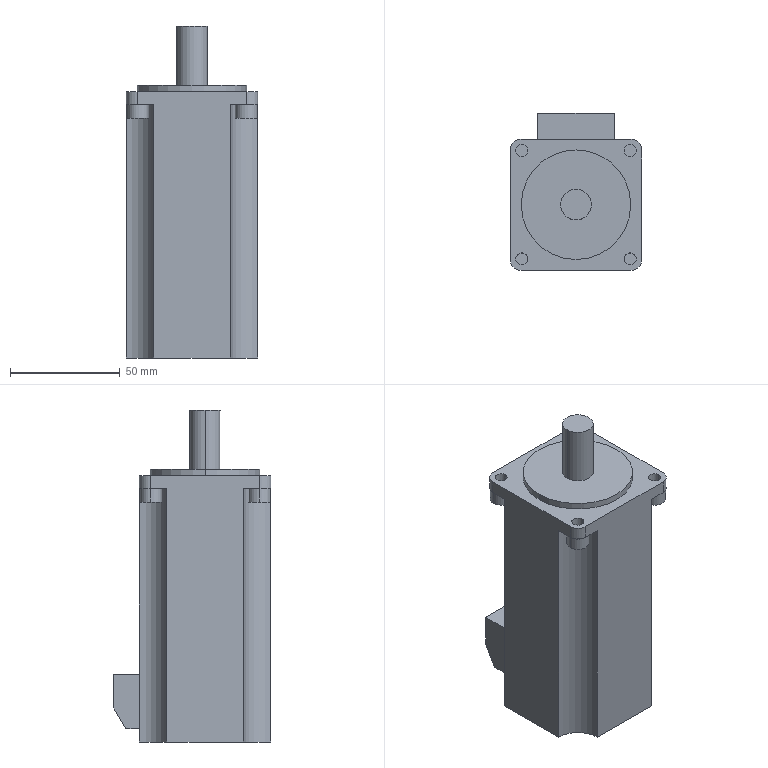Part | SolidWorks | features ICE 5, Chamfer 1, Extrusion 1, Fillet 1, HoleWzd 1 | 1 solid | 55 faces | box 60 x 72 x 151.5 mm | volume 401427 mm3 | cylinder 28 | plane 27 | commonest cylinder face diameters 10 x12 5.5 x8 25 x4 14 x2 50 x2
STEP:
#1=CARTESIAN_POINT('',(-29.749,24.749,-42.));
#2=VERTEX_POINT('',#1);
#3=CARTESIAN_POINT('',(-19.749,24.749,-42.));
#4=VERTEX_POINT('',#3);
#5=CARTESIAN_POINT('',(-24.749,24.749,-42.));
#6=DIRECTION('',(0.,0.,-1.));
#7=DIRECTION('',(-1.,0.,0.));
#8=AXIS2_PLACEMENT_3D('',#5,#6,#7);
#9=CIRCLE('',#8,5.);
#10=EDGE_CURVE('',#2,#4,#9,.T.);
#11=ORIENTED_EDGE('',*,*,#10,.F.);
#12=CARTESIAN_POINT('',(-29.749,24.749,-36.));
#13=VERTEX_POINT('',#12);
#14=CARTESIAN_POINT('',(-29.749,24.749,-42.));
#15=DIRECTION('',(0.,0.,1.));
#16=VECTOR('',#15,1000.);
#17=LINE('',#14,#16);
#18=EDGE_CURVE('',#2,#13,#17,.T.);
#19=ORIENTED_EDGE('',*,*,#18,.T.);
#20=CARTESIAN_POINT('',(-19.749,24.749,-36.));
#21=VERTEX_POINT('',#20);
#22=CARTESIAN_POINT('',(-24.749,24.749,-36.));
#23=DIRECTION('',(0.,0.,-1.));
#24=DIRECTION('',(-1.,0.,0.));
#25=AXIS2_PLACEMENT_3D('',#22,#23,#24);
#26=CIRCLE('',#25,5.);
#27=EDGE_CURVE('',#13,#21,#26,.T.);
#28=ORIENTED_EDGE('',*,*,#27,.T.);
#29=CARTESIAN_POINT('',(-19.749,24.749,-42.));
#30=DIRECTION('',(0.,0.,1.));
#31=VECTOR('',#30,1000.);
#32=LINE('',#29,#31);
#33=EDGE_CURVE('',#4,#21,#32,.T.);
#34=ORIENTED_EDGE('',*,*,#33,.F.);
#35=EDGE_LOOP('',(#11,#19,#28,#34));
#36=FACE_OUTER_BOUND('',#35,.T.);
#37=CARTESIAN_POINT('',(-24.749,24.749,-42.));
#38=DIRECTION('',(0.,0.,1.));
#39=DIRECTION('',(1.,0.,0.));
#40=AXIS2_PLACEMENT_3D('',#37,#38,#39);
#41=CYLINDRICAL_SURFACE('',#40,5.);
#42=ADVANCED_FACE('',(#36),#41,.T.);
#43=CARTESIAN_POINT('',(-29.749,-24.749,-42.));
#44=VERTEX_POINT('',#43);
#45=CARTESIAN_POINT('',(-19.749,-24.749,-42.));
#46=VERTEX_POINT('',#45);
#47=CARTESIAN_POINT('',(-24.749,-24.749,-42.));
#48=DIRECTION('',(0.,0.,-1.));
#49=DIRECTION('',(-1.,0.,0.));
#50=AXIS2_PLACEMENT_3D('',#47,#48,#49);
#51=CIRCLE('',#50,5.);
#52=EDGE_CURVE('',#44,#46,#51,.T.);
#53=ORIENTED_EDGE('',*,*,#52,.F.);
#54=CARTESIAN_POINT('',(-29.749,-24.749,-36.));
#55=VERTEX_POINT('',#54);
#56=CARTESIAN_POINT('',(-29.749,-24.749,-42.));
#57=DIRECTION('',(0.,0.,1.));
#58=VECTOR('',#57,1000.);
#59=LINE('',#56,#58);
#60=EDGE_CURVE('',#44,#55,#59,.T.);
#61=ORIENTED_EDGE('',*,*,#60,.T.);
#62=CARTESIAN_POINT('',(-19.749,-24.749,-36.));
#63=VERTEX_POINT('',#62);
#64=CARTESIAN_POINT('',(-24.749,-24.749,-36.));
#65=DIRECTION('',(0.,0.,-1.));
#66=DIRECTION('',(-1.,0.,0.));
#67=AXIS2_PLACEMENT_3D('',#64,#65,#66);
#68=CIRCLE('',#67,5.);
#69=EDGE_CURVE('',#55,#63,#68,.T.);
#70=ORIENTED_EDGE('',*,*,#69,.T.);
#71=CARTESIAN_POINT('',(-19.749,-24.749,-42.));
#72=DIRECTION('',(0.,0.,1.));
#73=VECTOR('',#72,1000.);
#74=LINE('',#71,#73);
#75=EDGE_CURVE('',#46,#63,#74,.T.);
#76=ORIENTED_EDGE('',*,*,#75,.F.);
#77=EDGE_LOOP('',(#53,#61,#70,#76));
#78=FACE_OUTER_BOUND('',#77,.T.);
#79=CARTESIAN_POINT('',(-24.749,-24.749,-42.));
#80=DIRECTION('',(0.,0.,1.));
#81=DIRECTION('',(1.,0.,0.));
#82=AXIS2_PLACEMENT_3D('',#79,#80,#81);
#83=CYLINDRICAL_SURFACE('',#82,5.);
#84=ADVANCED_FACE('',(#78),#83,.T.);
#85=CARTESIAN_POINT('',(19.749,-24.749,-42.));
#86=VERTEX_POINT('',#85);
#87=CARTESIAN_POINT('',(29.749,-24.749,-42.));
#88=VERTEX_POINT('',#87);
#89=CARTESIAN_POINT('',(24.749,-24.749,-42.));
#90=DIRECTION('',(0.,0.,-1.));
#91=DIRECTION('',(-1.,0.,0.));
#92=AXIS2_PLACEMENT_3D('',#89,#90,#91);
#93=CIRCLE('',#92,5.);
#94=EDGE_CURVE('',#86,#88,#93,.T.);
#95=ORIENTED_EDGE('',*,*,#94,.F.);
#96=CARTESIAN_POINT('',(19.749,-24.749,-36.));
#97=VERTEX_POINT('',#96);
#98=CARTESIAN_POINT('',(19.749,-24.749,-42.));
#99=DIRECTION('',(0.,0.,1.));
#100=VECTOR('',#99,1000.);
#101=LINE('',#98,#100);
#102=EDGE_CURVE('',#86,#97,#101,.T.);
#103=ORIENTED_EDGE('',*,*,#102,.T.);
#104=CARTESIAN_POINT('',(29.749,-24.749,-36.));
#105=VERTEX_POINT('',#104);
#106=CARTESIAN_POINT('',(24.749,-24.749,-36.));
#107=DIRECTION('',(0.,0.,-1.));
#108=DIRECTION('',(-1.,0.,0.));
#109=AXIS2_PLACEMENT_3D('',#106,#107,#108);
#110=CIRCLE('',#109,5.);
#111=EDGE_CURVE('',#97,#105,#110,.T.);
#112=ORIENTED_EDGE('',*,*,#111,.T.);
#113=CARTESIAN_POINT('',(29.749,-24.749,-42.));
#114=DIRECTION('',(0.,0.,1.));
#115=VECTOR('',#114,1000.);
#116=LINE('',#113,#115);
#117=EDGE_CURVE('',#88,#105,#116,.T.);
#118=ORIENTED_EDGE('',*,*,#117,.F.);
#119=EDGE_LOOP('',(#95,#103,#112,#118));
#120=FACE_OUTER_BOUND('',#119,.T.);
#121=CARTESIAN_POINT('',(24.749,-24.749,-42.));
#122=DIRECTION('',(0.,0.,1.));
#123=DIRECTION('',(1.,0.,0.));
#124=AXIS2_PLACEMENT_3D('',#121,#122,#123);
#125=CYLINDRICAL_SURFACE('',#124,5.);
#126=ADVANCED_FACE('',(#120),#125,.T.);
#127=CARTESIAN_POINT('',(19.749,24.749,-42.));
#128=VERTEX_POINT('',#127);
#129=CARTESIAN_POINT('',(29.749,24.749,-42.));
#130=VERTEX_POINT('',#129);
#131=CARTESIAN_POINT('',(24.749,24.749,-42.));
#132=DIRECTION('',(0.,0.,-1.));
#133=DIRECTION('',(-1.,0.,0.));
#134=AXIS2_PLACEMENT_3D('',#131,#132,#133);
#135=CIRCLE('',#134,5.);
#136=EDGE_CURVE('',#128,#130,#135,.T.);
#137=ORIENTED_EDGE('',*,*,#136,.F.);
#138=CARTESIAN_POINT('',(19.749,24.749,-36.));
#139=VERTEX_POINT('',#138);
#140=CARTESIAN_POINT('',(19.749,24.749,-42.));
#141=DIRECTION('',(0.,0.,1.));
#142=VECTOR('',#141,1000.);
#143=LINE('',#140,#142);
#144=EDGE_CURVE('',#128,#139,#143,.T.);
#145=ORIENTED_EDGE('',*,*,#144,.T.);
#146=CARTESIAN_POINT('',(29.749,24.749,-36.));
#147=VERTEX_POINT('',#146);
#148=CARTESIAN_POINT('',(24.749,24.749,-36.));
#149=DIRECTION('',(0.,0.,-1.));
#150=DIRECTION('',(-1.,0.,0.));
#151=AXIS2_PLACEMENT_3D('',#148,#149,#150);
#152=CIRCLE('',#151,5.);
#153=EDGE_CURVE('',#139,#147,#152,.T.);
#154=ORIENTED_EDGE('',*,*,#153,.T.);
#155=CARTESIAN_POINT('',(29.749,24.749,-42.));
#156=DIRECTION('',(0.,0.,1.));
#157=VECTOR('',#156,1000.);
#158=LINE('',#155,#157);
#159=EDGE_CURVE('',#130,#147,#158,.T.);
#160=ORIENTED_EDGE('',*,*,#159,.F.);
#161=EDGE_LOOP('',(#137,#145,#154,#160));
#162=FACE_OUTER_BOUND('',#161,.T.);
#163=CARTESIAN_POINT('',(24.749,24.749,-42.));
#164=DIRECTION('',(0.,0.,1.));
#165=DIRECTION('',(1.,0.,0.));
#166=AXIS2_PLACEMENT_3D('',#163,#164,#165);
#167=CYLINDRICAL_SURFACE('',#166,5.);
#168=ADVANCED_FACE('',(#162),#167,.T.);
#169=CARTESIAN_POINT('',(21.999,24.749,-36.));
#170=VERTEX_POINT('',#169);
#171=CARTESIAN_POINT('',(27.499,24.749,-36.));
#172=VERTEX_POINT('',#171);
#173=CARTESIAN_POINT('',(24.749,24.749,-36.));
#174=DIRECTION('',(0.,0.,1.));
#175=DIRECTION('',(-1.,0.,0.));
#176=AXIS2_PLACEMENT_3D('',#173,#174,#175);
#177=CIRCLE('',#176,2.75);
#178=EDGE_CURVE('',#170,#172,#177,.T.);
#179=ORIENTED_EDGE('',*,*,#178,.F.);
#180=CARTESIAN_POINT('',(21.999,24.749,-30.));
#181=VERTEX_POINT('',#180);
#182=CARTESIAN_POINT('',(21.999,24.749,-30.));
#183=DIRECTION('',(0.,0.,1.));
#184=VECTOR('',#183,1000.);
#185=LINE('',#182,#184);
#186=EDGE_CURVE('',#170,#181,#185,.T.);
#187=ORIENTED_EDGE('',*,*,#186,.T.);
#188=CARTESIAN_POINT('',(27.499,24.749,-30.));
#189=VERTEX_POINT('',#188);
#190=CARTESIAN_POINT('',(24.749,24.749,-30.));
#191=DIRECTION('',(0.,0.,1.));
#192=DIRECTION('',(1.,0.,0.));
#193=AXIS2_PLACEMENT_3D('',#190,#191,#192);
#194=CIRCLE('',#193,2.75);
#195=EDGE_CURVE('',#181,#189,#194,.T.);
#196=ORIENTED_EDGE('',*,*,#195,.T.);
#197=CARTESIAN_POINT('',(27.499,24.749,-30.));
#198=DIRECTION('',(0.,0.,1.));
#199=VECTOR('',#198,1000.);
#200=LINE('',#197,#199);
#201=EDGE_CURVE('',#172,#189,#200,.T.);
#202=ORIENTED_EDGE('',*,*,#201,.F.);
#203=EDGE_LOOP('',(#179,#187,#196,#202));
#204=FACE_OUTER_BOUND('',#203,.T.);
#205=CARTESIAN_POINT('',(24.749,24.749,-30.));
#206=DIRECTION('',(0.,0.,1.));
#207=DIRECTION('',(1.,0.,0.));
#208=AXIS2_PLACEMENT_3D('',#205,#206,#207);
#209=CYLINDRICAL_SURFACE('',#208,2.75);
#210=ADVANCED_FACE('',(#204),#209,.F.);
#211=CARTESIAN_POINT('',(-27.499,24.749,-36.));
#212=VERTEX_POINT('',#211);
#213=CARTESIAN_POINT('',(-21.999,24.749,-36.));
#214=VERTEX_POINT('',#213);
#215=CARTESIAN_POINT('',(-24.749,24.749,-36.));
#216=DIRECTION('',(0.,0.,1.));
#217=DIRECTION('',(-1.,0.,0.));
#218=AXIS2_PLACEMENT_3D('',#215,#216,#217);
#219=CIRCLE('',#218,2.75);
#220=EDGE_CURVE('',#212,#214,#219,.T.);
#221=ORIENTED_EDGE('',*,*,#220,.F.);
#222=CARTESIAN_POINT('',(-27.499,24.749,-30.));
#223=VERTEX_POINT('',#222);
#224=CARTESIAN_POINT('',(-27.499,24.749,-30.));
#225=DIRECTION('',(0.,0.,1.));
#226=VECTOR('',#225,1000.);
#227=LINE('',#224,#226);
#228=EDGE_CURVE('',#212,#223,#227,.T.);
#229=ORIENTED_EDGE('',*,*,#228,.T.);
#230=CARTESIAN_POINT('',(-21.999,24.749,-30.));
#231=VERTEX_POINT('',#230);
#232=CARTESIAN_POINT('',(-24.749,24.749,-30.));
#233=DIRECTION('',(0.,0.,1.));
#234=DIRECTION('',(1.,0.,0.));
#235=AXIS2_PLACEMENT_3D('',#232,#233,#234);
#236=CIRCLE('',#235,2.75);
#237=EDGE_CURVE('',#223,#231,#236,.T.);
#238=ORIENTED_EDGE('',*,*,#237,.T.);
#239=CARTESIAN_POINT('',(-21.999,24.749,-30.));
#240=DIRECTION('',(0.,0.,1.));
#241=VECTOR('',#240,1000.);
#242=LINE('',#239,#241);
#243=EDGE_CURVE('',#214,#231,#242,.T.);
#244=ORIENTED_EDGE('',*,*,#243,.F.);
#245=EDGE_LOOP('',(#221,#229,#238,#244));
#246=FACE_OUTER_BOUND('',#245,.T.);
#247=CARTESIAN_POINT('',(-24.749,24.749,-30.));
#248=DIRECTION('',(0.,0.,1.));
#249=DIRECTION('',(1.,0.,0.));
#250=AXIS2_PLACEMENT_3D('',#247,#248,#249);
#251=CYLINDRICAL_SURFACE('',#250,2.75);
#252=ADVANCED_FACE('',(#246),#251,.F.);
#253=CARTESIAN_POINT('',(21.999,-24.749,-36.));
#254=VERTEX_POINT('',#253);
#255=CARTESIAN_POINT('',(27.499,-24.749,-36.));
#256=VERTEX_POINT('',#255);
#257=CARTESIAN_POINT('',(24.749,-24.749,-36.));
#258=DIRECTION('',(0.,0.,1.));
#259=DIRECTION('',(-1.,0.,0.));
#260=AXIS2_PLACEMENT_3D('',#257,#258,#259);
#261=CIRCLE('',#260,2.75);
#262=EDGE_CURVE('',#254,#256,#261,.T.);
#263=ORIENTED_EDGE('',*,*,#262,.F.);
#264=CARTESIAN_POINT('',(21.999,-24.749,-30.));
#265=VERTEX_POINT('',#264);
#266=CARTESIAN_POINT('',(21.999,-24.749,-30.));
#267=DIRECTION('',(0.,0.,1.));
#268=VECTOR('',#267,1000.);
#269=LINE('',#266,#268);
#270=EDGE_CURVE('',#254,#265,#269,.T.);
#271=ORIENTED_EDGE('',*,*,#270,.T.);
#272=CARTESIAN_POINT('',(27.499,-24.749,-30.));
#273=VERTEX_POINT('',#272);
#274=CARTESIAN_POINT('',(24.749,-24.749,-30.));
#275=DIRECTION('',(0.,0.,1.));
#276=DIRECTION('',(1.,0.,0.));
#277=AXIS2_PLACEMENT_3D('',#274,#275,#276);
#278=CIRCLE('',#277,2.75);
#279=EDGE_CURVE('',#265,#273,#278,.T.);
#280=ORIENTED_EDGE('',*,*,#279,.T.);
#281=CARTESIAN_POINT('',(27.499,-24.749,-30.));
#282=DIRECTION('',(0.,0.,1.));
#283=VECTOR('',#282,1000.);
#284=LINE('',#281,#283);
#285=EDGE_CURVE('',#256,#273,#284,.T.);
#286=ORIENTED_EDGE('',*,*,#285,.F.);
#287=EDGE_LOOP('',(#263,#271,#280,#286));
#288=FACE_OUTER_BOUND('',#287,.T.);
#289=CARTESIAN_POINT('',(24.749,-24.749,-30.));
#290=DIRECTION('',(0.,0.,1.));
#291=DIRECTION('',(1.,0.,0.));
#292=AXIS2_PLACEMENT_3D('',#289,#290,#291);
#293=CYLINDRICAL_SURFACE('',#292,2.75);
#294=ADVANCED_FACE('',(#288),#293,.F.);
#295=CARTESIAN_POINT('',(-27.499,-24.749,-36.));
#296=VERTEX_POINT('',#295);
#297=CARTESIAN_POINT('',(-21.999,-24.749,-36.));
#298=VERTEX_POINT('',#297);
#299=CARTESIAN_POINT('',(-24.749,-24.749,-36.));
#300=DIRECTION('',(0.,0.,1.));
#301=DIRECTION('',(-1.,0.,0.));
#302=AXIS2_PLACEMENT_3D('',#299,#300,#301);
#303=CIRCLE('',#302,2.75);
#304=EDGE_CURVE('',#296,#298,#303,.T.);
#305=ORIENTED_EDGE('',*,*,#304,.F.);
#306=CARTESIAN_POINT('',(-27.499,-24.749,-30.));
#307=VERTEX_POINT('',#306);
#308=CARTESIAN_POINT('',(-27.499,-24.749,-30.));
#309=DIRECTION('',(0.,0.,1.));
#310=VECTOR('',#309,1000.);
#311=LINE('',#308,#310);
#312=EDGE_CURVE('',#296,#307,#311,.T.);
#313=ORIENTED_EDGE('',*,*,#312,.T.);
#314=CARTESIAN_POINT('',(-21.999,-24.749,-30.));
#315=VERTEX_POINT('',#314);
#316=CARTESIAN_POINT('',(-24.749,-24.749,-30.));
#317=DIRECTION('',(0.,0.,1.));
#318=DIRECTION('',(1.,0.,0.));
#319=AXIS2_PLACEMENT_3D('',#316,#317,#318);
#320=CIRCLE('',#319,2.75);
#321=EDGE_CURVE('',#307,#315,#320,.T.);
#322=ORIENTED_EDGE('',*,*,#321,.T.);
#323=CARTESIAN_POINT('',(-21.999,-24.749,-30.));
#324=DIRECTION('',(0.,0.,1.));
#325=VECTOR('',#324,1000.);
#326=LINE('',#323,#325);
#327=EDGE_CURVE('',#298,#315,#326,.T.);
#328=ORIENTED_EDGE('',*,*,#327,.F.);
#329=EDGE_LOOP('',(#305,#313,#322,#328));
#330=FACE_OUTER_BOUND('',#329,.T.);
#331=CARTESIAN_POINT('',(-24.749,-24.749,-30.));
#332=DIRECTION('',(0.,0.,1.));
#333=DIRECTION('',(1.,0.,0.));
#334=AXIS2_PLACEMENT_3D('',#331,#332,#333);
#335=CYLINDRICAL_SURFACE('',#334,2.75);
#336=ADVANCED_FACE('',(#330),#335,.F.);
#337=CARTESIAN_POINT('',(-25.,0.,-27.));
#338=VERTEX_POINT('',#337);
#339=CARTESIAN_POINT('',(25.,0.,-27.));
#340=VERTEX_POINT('',#339);
#341=CARTESIAN_POINT('',(0.,0.,-27.));
#342=DIRECTION('',(0.,0.,-1.));
#343=DIRECTION('',(-1.,0.,0.));
#344=AXIS2_PLACEMENT_3D('',#341,#342,#343);
#345=CIRCLE('',#344,25.);
#346=EDGE_CURVE('',#338,#340,#345,.T.);
#347=ORIENTED_EDGE('',*,*,#346,.T.);
#348=CARTESIAN_POINT('',(25.,0.,-30.));
#349=VERTEX_POINT('',#348);
#350=CARTESIAN_POINT('',(25.,0.,-27.));
#351=DIRECTION('',(0.,0.,-1.));
#352=VECTOR('',#351,1000.);
#353=LINE('',#350,#352);
#354=EDGE_CURVE('',#340,#349,#353,.T.);
#355=ORIENTED_EDGE('',*,*,#354,.T.);
#356=CARTESIAN_POINT('',(-25.,0.,-30.));
#357=VERTEX_POINT('',#356);
#358=CARTESIAN_POINT('',(0.,0.,-30.));
#359=DIRECTION('',(0.,0.,-1.));
#360=DIRECTION('',(-1.,0.,0.));
#361=AXIS2_PLACEMENT_3D('',#358,#359,#360);
#362=CIRCLE('',#361,25.);
#363=EDGE_CURVE('',#357,#349,#362,.T.);
#364=ORIENTED_EDGE('',*,*,#363,.F.);
#365=CARTESIAN_POINT('',(-25.,0.,-27.));
#366=DIRECTION('',(0.,0.,-1.));
#367=VECTOR('',#366,1000.);
#368=LINE('',#365,#367);
#369=EDGE_CURVE('',#338,#357,#368,.T.);
#370=ORIENTED_EDGE('',*,*,#369,.F.);
#371=EDGE_LOOP('',(#347,#355,#364,#370));
#372=FACE_OUTER_BOUND('',#371,.T.);
#373=CARTESIAN_POINT('',(0.,0.,-27.));
#374=DIRECTION('',(0.,0.,-1.));
#375=DIRECTION('',(-1.,0.,0.));
#376=AXIS2_PLACEMENT_3D('',#373,#374,#375);
#377=CYLINDRICAL_SURFACE('',#376,25.);
#378=ADVANCED_FACE('',(#372),#377,.T.);
#379=CARTESIAN_POINT('',(7.,0.,-27.));
#380=VERTEX_POINT('',#379);
#381=CARTESIAN_POINT('',(-7.,0.,-27.));
#382=VERTEX_POINT('',#381);
#383=CARTESIAN_POINT('',(0.,0.,-27.));
#384=DIRECTION('',(0.,0.,1.));
#385=DIRECTION('',(-1.,0.,0.));
#386=AXIS2_PLACEMENT_3D('',#383,#384,#385);
#387=CIRCLE('',#386,7.);
#388=EDGE_CURVE('',#380,#382,#387,.T.);
#389=ORIENTED_EDGE('',*,*,#388,.T.);
#390=CARTESIAN_POINT('',(-7.,0.,0.));
#391=VERTEX_POINT('',#390);
#392=CARTESIAN_POINT('',(-7.,0.,-30.));
#393=DIRECTION('',(0.,0.,1.));
#394=VECTOR('',#393,1000.);
#395=LINE('',#392,#394);
#396=EDGE_CURVE('',#382,#391,#395,.T.);
#397=ORIENTED_EDGE('',*,*,#396,.T.);
#398=CARTESIAN_POINT('',(7.,0.,0.));
#399=VERTEX_POINT('',#398);
#400=CARTESIAN_POINT('',(0.,0.,0.));
#401=DIRECTION('',(0.,0.,1.));
#402=DIRECTION('',(1.,0.,0.));
#403=AXIS2_PLACEMENT_3D('',#400,#401,#402);
#404=CIRCLE('',#403,7.);
#405=EDGE_CURVE('',#399,#391,#404,.T.);
#406=ORIENTED_EDGE('',*,*,#405,.F.);
#407=CARTESIAN_POINT('',(7.,0.,-30.));
#408=DIRECTION('',(0.,0.,1.));
#409=VECTOR('',#408,1000.);
#410=LINE('',#407,#409);
#411=EDGE_CURVE('',#380,#399,#410,.T.);
#412=ORIENTED_EDGE('',*,*,#411,.F.);
#413=EDGE_LOOP('',(#389,#397,#406,#412));
#414=FACE_OUTER_BOUND('',#413,.T.);
#415=CARTESIAN_POINT('',(0.,0.,-30.));
#416=DIRECTION('',(0.,0.,1.));
#417=DIRECTION('',(1.,0.,0.));
#418=AXIS2_PLACEMENT_3D('',#415,#416,#417);
#419=CYLINDRICAL_SURFACE('',#418,7.);
#420=ADVANCED_FACE('',(#414),#419,.T.);
#421=CARTESIAN_POINT('',(-30.,17.5,-36.));
#422=VERTEX_POINT('',#421);
#423=CARTESIAN_POINT('',(-30.,25.,-36.));
#424=VERTEX_POINT('',#423);
#425=CARTESIAN_POINT('',(-30.,30.,-36.));
#426=DIRECTION('',(0.,1.,0.));
#427=VECTOR('',#426,1000.);
#428=LINE('',#425,#427);
#429=EDGE_CURVE('',#422,#424,#428,.T.);
#430=ORIENTED_EDGE('',*,*,#429,.T.);
#431=CARTESIAN_POINT('',(-25.,30.,-36.));
#432=VERTEX_POINT('',#431);
#433=CARTESIAN_POINT('',(-25.,25.,-36.));
#434=DIRECTION('',(0.,0.,-1.));
#435=DIRECTION('',(-1.,0.,0.));
#436=AXIS2_PLACEMENT_3D('',#433,#434,#435);
#437=CIRCLE('',#436,5.);
#438=EDGE_CURVE('',#424,#432,#437,.T.);
#439=ORIENTED_EDGE('',*,*,#438,.T.);
#440=CARTESIAN_POINT('',(-17.5,30.,-36.));
#441=VERTEX_POINT('',#440);
#442=CARTESIAN_POINT('',(30.,30.,-36.));
#443=DIRECTION('',(1.,0.,0.));
#444=VECTOR('',#443,1000.);
#445=LINE('',#442,#444);
#446=EDGE_CURVE('',#432,#441,#445,.T.);
#447=ORIENTED_EDGE('',*,*,#446,.T.);
#448=CARTESIAN_POINT('',(-30.,30.,-36.));
#449=DIRECTION('',(0.,0.,1.));
#450=DIRECTION('',(-1.,0.,0.));
#451=AXIS2_PLACEMENT_3D('',#448,#449,#450);
#452=CIRCLE('',#451,12.5);
#453=EDGE_CURVE('',#422,#441,#452,.T.);
#454=ORIENTED_EDGE('',*,*,#453,.F.);
#455=EDGE_LOOP('',(#430,#439,#447,#454));
#456=FACE_OUTER_BOUND('',#455,.T.);
#457=CARTESIAN_POINT('',(-24.749,24.749,-36.));
#458=DIRECTION('',(0.,0.,-1.));
#459=DIRECTION('',(-1.,0.,0.));
#460=AXIS2_PLACEMENT_3D('',#457,#458,#459);
#461=CIRCLE('',#460,5.);
#462=EDGE_CURVE('',#21,#13,#461,.T.);
#463=ORIENTED_EDGE('',*,*,#462,.F.);
#464=ORIENTED_EDGE('',*,*,#27,.F.);
#465=EDGE_LOOP('',(#463,#464));
#466=FACE_BOUND('',#465,.T.);
#467=CARTESIAN_POINT('',(0.,0.,-36.));
#468=DIRECTION('',(0.,0.,-1.));
#469=DIRECTION('',(-1.,0.,0.));
#470=AXIS2_PLACEMENT_3D('',#467,#468,#469);
#471=PLANE('',#470);
#472=ADVANCED_FACE('',(#456,#466),#471,.T.);
#473=CARTESIAN_POINT('',(-17.5,-30.,-36.));
#474=VERTEX_POINT('',#473);
#475=CARTESIAN_POINT('',(-25.,-30.,-36.));
#476=VERTEX_POINT('',#475);
#477=CARTESIAN_POINT('',(30.,-30.,-36.));
#478=DIRECTION('',(-1.,0.,0.));
#479=VECTOR('',#478,1000.);
#480=LINE('',#477,#479);
#481=EDGE_CURVE('',#474,#476,#480,.T.);
#482=ORIENTED_EDGE('',*,*,#481,.T.);
#483=CARTESIAN_POINT('',(-30.,-25.,-36.));
#484=VERTEX_POINT('',#483);
#485=CARTESIAN_POINT('',(-25.,-25.,-36.));
#486=DIRECTION('',(0.,0.,-1.));
#487=DIRECTION('',(-1.,0.,0.));
#488=AXIS2_PLACEMENT_3D('',#485,#486,#487);
#489=CIRCLE('',#488,5.);
#490=EDGE_CURVE('',#476,#484,#489,.T.);
#491=ORIENTED_EDGE('',*,*,#490,.T.);
#492=CARTESIAN_POINT('',(-30.,-17.5,-36.));
#493=VERTEX_POINT('',#492);
#494=CARTESIAN_POINT('',(-30.,30.,-36.));
#495=DIRECTION('',(0.,1.,0.));
#496=VECTOR('',#495,1000.);
#497=LINE('',#494,#496);
#498=EDGE_CURVE('',#484,#493,#497,.T.);
#499=ORIENTED_EDGE('',*,*,#498,.T.);
#500=CARTESIAN_POINT('',(-30.,-30.,-36.));
#501=DIRECTION('',(0.,0.,1.));
#502=DIRECTION('',(-1.,0.,0.));
#503=AXIS2_PLACEMENT_3D('',#500,#501,#502);
#504=CIRCLE('',#503,12.5);
#505=EDGE_CURVE('',#474,#493,#504,.T.);
#506=ORIENTED_EDGE('',*,*,#505,.F.);
#507=EDGE_LOOP('',(#482,#491,#499,#506));
#508=FACE_OUTER_BOUND('',#507,.T.);
#509=CARTESIAN_POINT('',(-24.749,-24.749,-36.));
#510=DIRECTION('',(0.,0.,-1.));
#511=DIRECTION('',(-1.,0.,0.));
#512=AXIS2_PLACEMENT_3D('',#509,#510,#511);
#513=CIRCLE('',#512,5.);
#514=EDGE_CURVE('',#63,#55,#513,.T.);
#515=ORIENTED_EDGE('',*,*,#514,.F.);
#516=ORIENTED_EDGE('',*,*,#69,.F.);
#517=EDGE_LOOP('',(#515,#516));
#518=FACE_BOUND('',#517,.T.);
#519=CARTESIAN_POINT('',(0.,0.,-36.));
#520=DIRECTION('',(0.,0.,-1.));
#521=DIRECTION('',(-1.,0.,0.));
#522=AXIS2_PLACEMENT_3D('',#519,#520,#521);
#523=PLANE('',#522);
#524=ADVANCED_FACE('',(#508,#518),#523,.T.);
#525=CARTESIAN_POINT('',(30.,-17.5,-36.));
#526=VERTEX_POINT('',#525);
#527=CARTESIAN_POINT('',(30.,-25.,-36.));
#528=VERTEX_POINT('',#527);
#529=CARTESIAN_POINT('',(30.,30.,-36.));
#530=DIRECTION('',(0.,-1.,0.));
#531=VECTOR('',#530,1000.);
#532=LINE('',#529,#531);
#533=EDGE_CURVE('',#526,#528,#532,.T.);
#534=ORIENTED_EDGE('',*,*,#533,.T.);
#535=CARTESIAN_POINT('',(25.,-30.,-36.));
#536=VERTEX_POINT('',#535);
#537=CARTESIAN_POINT('',(25.,-25.,-36.));
#538=DIRECTION('',(0.,0.,-1.));
#539=DIRECTION('',(-1.,0.,0.));
#540=AXIS2_PLACEMENT_3D('',#537,#538,#539);
#541=CIRCLE('',#540,5.);
#542=EDGE_CURVE('',#528,#536,#541,.T.);
#543=ORIENTED_EDGE('',*,*,#542,.T.);
#544=CARTESIAN_POINT('',(17.5,-30.,-36.));
#545=VERTEX_POINT('',#544);
#546=CARTESIAN_POINT('',(30.,-30.,-36.));
#547=DIRECTION('',(-1.,0.,0.));
#548=VECTOR('',#547,1000.);
#549=LINE('',#546,#548);
#550=EDGE_CURVE('',#536,#545,#549,.T.);
#551=ORIENTED_EDGE('',*,*,#550,.T.);
#552=CARTESIAN_POINT('',(30.,-30.,-36.));
#553=DIRECTION('',(0.,0.,1.));
#554=DIRECTION('',(-1.,0.,0.));
#555=AXIS2_PLACEMENT_3D('',#552,#553,#554);
#556=CIRCLE('',#555,12.5);
#557=EDGE_CURVE('',#526,#545,#556,.T.);
#558=ORIENTED_EDGE('',*,*,#557,.F.);
#559=EDGE_LOOP('',(#534,#543,#551,#558));
#560=FACE_OUTER_BOUND('',#559,.T.);
#561=CARTESIAN_POINT('',(24.749,-24.749,-36.));
#562=DIRECTION('',(0.,0.,-1.));
#563=DIRECTION('',(-1.,0.,0.));
#564=AXIS2_PLACEMENT_3D('',#561,#562,#563);
#565=CIRCLE('',#564,5.);
#566=EDGE_CURVE('',#105,#97,#565,.T.);
#567=ORIENTED_EDGE('',*,*,#566,.F.);
#568=ORIENTED_EDGE('',*,*,#111,.F.);
#569=EDGE_LOOP('',(#567,#568));
#570=FACE_BOUND('',#569,.T.);
#571=CARTESIAN_POINT('',(0.,0.,-36.));
#572=DIRECTION('',(0.,0.,-1.));
#573=DIRECTION('',(-1.,0.,0.));
#574=AXIS2_PLACEMENT_3D('',#571,#572,#573);
#575=PLANE('',#574);
#576=ADVANCED_FACE('',(#560,#570),#575,.T.);
#577=CARTESIAN_POINT('',(17.5,30.,-36.));
#578=VERTEX_POINT('',#577);
#579=CARTESIAN_POINT('',(25.,30.,-36.));
#580=VERTEX_POINT('',#579);
#581=CARTESIAN_POINT('',(30.,30.,-36.));
#582=DIRECTION('',(1.,0.,0.));
#583=VECTOR('',#582,1000.);
#584=LINE('',#581,#583);
#585=EDGE_CURVE('',#578,#580,#584,.T.);
#586=ORIENTED_EDGE('',*,*,#585,.T.);
#587=CARTESIAN_POINT('',(30.,25.,-36.));
#588=VERTEX_POINT('',#587);
#589=CARTESIAN_POINT('',(25.,25.,-36.));
#590=DIRECTION('',(0.,0.,-1.));
#591=DIRECTION('',(-1.,0.,0.));
#592=AXIS2_PLACEMENT_3D('',#589,#590,#591);
#593=CIRCLE('',#592,5.);
#594=EDGE_CURVE('',#580,#588,#593,.T.);
#595=ORIENTED_EDGE('',*,*,#594,.T.);
#596=CARTESIAN_POINT('',(30.,17.5,-36.));
#597=VERTEX_POINT('',#596);
#598=CARTESIAN_POINT('',(30.,30.,-36.));
#599=DIRECTION('',(0.,-1.,0.));
#600=VECTOR('',#599,1000.);
#601=LINE('',#598,#600);
#602=EDGE_CURVE('',#588,#597,#601,.T.);
#603=ORIENTED_EDGE('',*,*,#602,.T.);
#604=CARTESIAN_POINT('',(30.,30.,-36.));
#605=DIRECTION('',(0.,0.,1.));
#606=DIRECTION('',(-1.,0.,0.));
#607=AXIS2_PLACEMENT_3D('',#604,#605,#606);
#608=CIRCLE('',#607,12.5);
#609=EDGE_CURVE('',#578,#597,#608,.T.);
#610=ORIENTED_EDGE('',*,*,#609,.F.);
#611=EDGE_LOOP('',(#586,#595,#603,#610));
#612=FACE_OUTER_BOUND('',#611,.T.);
#613=CARTESIAN_POINT('',(24.749,24.749,-36.));
#614=DIRECTION('',(0.,0.,-1.));
#615=DIRECTION('',(-1.,0.,0.));
#616=AXIS2_PLACEMENT_3D('',#613,#614,#615);
#617=CIRCLE('',#616,5.);
#618=EDGE_CURVE('',#147,#139,#617,.T.);
#619=ORIENTED_EDGE('',*,*,#618,.F.);
#620=ORIENTED_EDGE('',*,*,#153,.F.);
#621=EDGE_LOOP('',(#619,#620));
#622=FACE_BOUND('',#621,.T.);
#623=CARTESIAN_POINT('',(0.,0.,-36.));
#624=DIRECTION('',(0.,0.,-1.));
#625=DIRECTION('',(-1.,0.,0.));
#626=AXIS2_PLACEMENT_3D('',#623,#624,#625);
#627=PLANE('',#626);
#628=ADVANCED_FACE('',(#612,#622),#627,.T.);
#629=CARTESIAN_POINT('',(17.5,30.,-145.5));
#630=VERTEX_POINT('',#629);
#631=CARTESIAN_POINT('',(-17.5,30.,-145.5));
#632=VERTEX_POINT('',#631);
#633=CARTESIAN_POINT('',(-17.5,30.,-145.5));
#634=DIRECTION('',(-1.,0.,0.));
#635=VECTOR('',#634,1000.);
#636=LINE('',#633,#635);
#637=EDGE_CURVE('',#630,#632,#636,.T.);
#638=ORIENTED_EDGE('',*,*,#637,.F.);
#639=CARTESIAN_POINT('',(17.5,30.,-151.5));
#640=VERTEX_POINT('',#639);
#641=CARTESIAN_POINT('',(17.5,30.,-151.5));
#642=DIRECTION('',(0.,0.,1.));
#643=VECTOR('',#642,1000.);
#644=LINE('',#641,#643);
#645=EDGE_CURVE('',#640,#630,#644,.T.);
#646=ORIENTED_EDGE('',*,*,#645,.F.);
#647=CARTESIAN_POINT('',(-17.5,30.,-151.5));
#648=VERTEX_POINT('',#647);
#649=CARTESIAN_POINT('',(-17.5,30.,-151.5));
#650=DIRECTION('',(1.,0.,0.));
#651=VECTOR('',#650,1000.);
#652=LINE('',#649,#651);
#653=EDGE_CURVE('',#648,#640,#652,.T.);
#654=ORIENTED_EDGE('',*,*,#653,.F.);
#655=CARTESIAN_POINT('',(-17.5,30.,-151.5));
#656=DIRECTION('',(0.,0.,1.));
#657=VECTOR('',#656,1000.);
#658=LINE('',#655,#657);
#659=EDGE_CURVE('',#648,#632,#658,.T.);
#660=ORIENTED_EDGE('',*,*,#659,.T.);
#661=EDGE_LOOP('',(#638,#646,#654,#660));
#662=FACE_OUTER_BOUND('',#661,.T.);
#663=CARTESIAN_POINT('',(30.,30.,-36.));
#664=DIRECTION('',(0.,-1.,0.));
#665=DIRECTION('',(0.,0.,-1.));
#666=AXIS2_PLACEMENT_3D('',#663,#664,#665);
#667=PLANE('',#666);
#668=ADVANCED_FACE('',(#662),#667,.F.);
#669=ORIENTED_EDGE('',*,*,#446,.F.);
#670=CARTESIAN_POINT('',(-25.,30.,-30.));
#671=VERTEX_POINT('',#670);
#672=CARTESIAN_POINT('',(-25.,30.,-36.));
#673=DIRECTION('',(0.,0.,1.));
#674=VECTOR('',#673,1000.);
#675=LINE('',#672,#674);
#676=EDGE_CURVE('',#432,#671,#675,.T.);
#677=ORIENTED_EDGE('',*,*,#676,.T.);
#678=CARTESIAN_POINT('',(25.,30.,-30.));
#679=VERTEX_POINT('',#678);
#680=CARTESIAN_POINT('',(30.,30.,-30.));
#681=DIRECTION('',(1.,0.,0.));
#682=VECTOR('',#681,1000.);
#683=LINE('',#680,#682);
#684=EDGE_CURVE('',#671,#679,#683,.T.);
#685=ORIENTED_EDGE('',*,*,#684,.T.);
#686=CARTESIAN_POINT('',(25.,30.,-36.));
#687=DIRECTION('',(0.,0.,-1.));
#688=VECTOR('',#687,1000.);
#689=LINE('',#686,#688);
#690=EDGE_CURVE('',#679,#580,#689,.T.);
#691=ORIENTED_EDGE('',*,*,#690,.T.);
#692=ORIENTED_EDGE('',*,*,#585,.F.);
#693=CARTESIAN_POINT('',(17.5,30.,-120.5));
#694=VERTEX_POINT('',#693);
#695=CARTESIAN_POINT('',(17.5,30.,-151.5));
#696=DIRECTION('',(0.,0.,1.));
#697=VECTOR('',#696,1000.);
#698=LINE('',#695,#697);
#699=EDGE_CURVE('',#694,#578,#698,.T.);
#700=ORIENTED_EDGE('',*,*,#699,.F.);
#701=CARTESIAN_POINT('',(-17.5,30.,-120.5));
#702=VERTEX_POINT('',#701);
#703=CARTESIAN_POINT('',(-17.5,30.,-120.5));
#704=DIRECTION('',(1.,0.,0.));
#705=VECTOR('',#704,1000.);
#706=LINE('',#703,#705);
#707=EDGE_CURVE('',#702,#694,#706,.T.);
#708=ORIENTED_EDGE('',*,*,#707,.F.);
#709=CARTESIAN_POINT('',(-17.5,30.,-151.5));
#710=DIRECTION('',(0.,0.,1.));
#711=VECTOR('',#710,1000.);
#712=LINE('',#709,#711);
#713=EDGE_CURVE('',#702,#441,#712,.T.);
#714=ORIENTED_EDGE('',*,*,#713,.T.);
#715=EDGE_LOOP('',(#669,#677,#685,#691,#692,#700,#708,#714));
#716=FACE_OUTER_BOUND('',#715,.T.);
#717=CARTESIAN_POINT('',(30.,30.,-36.));
#718=DIRECTION('',(0.,-1.,0.));
#719=DIRECTION('',(0.,0.,-1.));
#720=AXIS2_PLACEMENT_3D('',#717,#718,#719);
#721=PLANE('',#720);
#722=ADVANCED_FACE('',(#716),#721,.F.);
#723=ORIENTED_EDGE('',*,*,#396,.F.);
#724=CARTESIAN_POINT('',(0.,0.,-27.));
#725=DIRECTION('',(0.,0.,1.));
#726=DIRECTION('',(-1.,0.,0.));
#727=AXIS2_PLACEMENT_3D('',#724,#725,#726);
#728=CIRCLE('',#727,7.);
#729=EDGE_CURVE('',#382,#380,#728,.T.);
#730=ORIENTED_EDGE('',*,*,#729,.T.);
#731=ORIENTED_EDGE('',*,*,#411,.T.);
#732=CARTESIAN_POINT('',(0.,0.,0.));
#733=DIRECTION('',(0.,0.,1.));
#734=DIRECTION('',(1.,0.,0.));
#735=AXIS2_PLACEMENT_3D('',#732,#733,#734);
#736=CIRCLE('',#735,7.);
#737=EDGE_CURVE('',#391,#399,#736,.T.);
#738=ORIENTED_EDGE('',*,*,#737,.F.);
#739=EDGE_LOOP('',(#723,#730,#731,#738));
#740=FACE_OUTER_BOUND('',#739,.T.);
#741=CARTESIAN_POINT('',(0.,0.,-30.));
#742=DIRECTION('',(0.,0.,1.));
#743=DIRECTION('',(1.,0.,0.));
#744=AXIS2_PLACEMENT_3D('',#741,#742,#743);
#745=CYLINDRICAL_SURFACE('',#744,7.);
#746=ADVANCED_FACE('',(#740),#745,.T.);
#747=ORIENTED_EDGE('',*,*,#405,.T.);
#748=ORIENTED_EDGE('',*,*,#737,.T.);
#749=EDGE_LOOP('',(#747,#748));
#750=FACE_OUTER_BOUND('',#749,.T.);
#751=CARTESIAN_POINT('',(0.,0.,0.));
#752=DIRECTION('',(0.,0.,1.));
#753=DIRECTION('',(1.,0.,0.));
#754=AXIS2_PLACEMENT_3D('',#751,#752,#753);
#755=PLANE('',#754);
#756=ADVANCED_FACE('',(#750),#755,.T.);
#757=ORIENTED_EDGE('',*,*,#354,.F.);
#758=CARTESIAN_POINT('',(0.,0.,-27.));
#759=DIRECTION('',(0.,0.,-1.));
#760=DIRECTION('',(-1.,0.,0.));
#761=AXIS2_PLACEMENT_3D('',#758,#759,#760);
#762=CIRCLE('',#761,25.);
#763=EDGE_CURVE('',#340,#338,#762,.T.);
#764=ORIENTED_EDGE('',*,*,#763,.T.);
#765=ORIENTED_EDGE('',*,*,#369,.T.);
#766=CARTESIAN_POINT('',(0.,0.,-30.));
#767=DIRECTION('',(0.,0.,-1.));
#768=DIRECTION('',(-1.,0.,0.));
#769=AXIS2_PLACEMENT_3D('',#766,#767,#768);
#770=CIRCLE('',#769,25.);
#771=EDGE_CURVE('',#349,#357,#770,.T.);
#772=ORIENTED_EDGE('',*,*,#771,.F.);
#773=EDGE_LOOP('',(#757,#764,#765,#772));
#774=FACE_OUTER_BOUND('',#773,.T.);
#775=CARTESIAN_POINT('',(0.,0.,-27.));
#776=DIRECTION('',(0.,0.,-1.));
#777=DIRECTION('',(-1.,0.,0.));
#778=AXIS2_PLACEMENT_3D('',#775,#776,#777);
#779=CYLINDRICAL_SURFACE('',#778,25.);
#780=ADVANCED_FACE('',(#774),#779,.T.);
#781=ORIENTED_EDGE('',*,*,#388,.F.);
#782=ORIENTED_EDGE('',*,*,#729,.F.);
#783=EDGE_LOOP('',(#781,#782));
#784=FACE_BOUND('',#783,.T.);
#785=ORIENTED_EDGE('',*,*,#346,.F.);
#786=ORIENTED_EDGE('',*,*,#763,.F.);
#787=EDGE_LOOP('',(#785,#786));
#788=FACE_OUTER_BOUND('',#787,.T.);
#789=CARTESIAN_POINT('',(0.,0.,-27.));
#790=DIRECTION('',(0.,0.,-1.));
#791=DIRECTION('',(-1.,0.,0.));
#792=AXIS2_PLACEMENT_3D('',#789,#790,#791);
#793=PLANE('',#792);
#794=ADVANCED_FACE('',(#784,#788),#793,.F.);
#795=ORIENTED_EDGE('',*,*,#498,.F.);
#796=CARTESIAN_POINT('',(-30.,-25.,-30.));
#797=VERTEX_POINT('',#796);
#798=CARTESIAN_POINT('',(-30.,-25.,-36.));
#799=DIRECTION('',(0.,0.,1.));
#800=VECTOR('',#799,1000.);
#801=LINE('',#798,#800);
#802=EDGE_CURVE('',#484,#797,#801,.T.);
#803=ORIENTED_EDGE('',*,*,#802,.T.);
#804=CARTESIAN_POINT('',(-30.,25.,-30.));
#805=VERTEX_POINT('',#804);
#806=CARTESIAN_POINT('',(-30.,30.,-30.));
#807=DIRECTION('',(0.,1.,0.));
#808=VECTOR('',#807,1000.);
#809=LINE('',#806,#808);
#810=EDGE_CURVE('',#797,#805,#809,.T.);
#811=ORIENTED_EDGE('',*,*,#810,.T.);
#812=CARTESIAN_POINT('',(-30.,25.,-36.));
#813=DIRECTION('',(0.,0.,-1.));
#814=VECTOR('',#813,1000.);
#815=LINE('',#812,#814);
#816=EDGE_CURVE('',#805,#424,#815,.T.);
#817=ORIENTED_EDGE('',*,*,#816,.T.);
#818=ORIENTED_EDGE('',*,*,#429,.F.);
#819=CARTESIAN_POINT('',(-30.,17.5,-151.5));
#820=VERTEX_POINT('',#819);
#821=CARTESIAN_POINT('',(-30.,17.5,-151.5));
#822=DIRECTION('',(0.,0.,1.));
#823=VECTOR('',#822,1000.);
#824=LINE('',#821,#823);
#825=EDGE_CURVE('',#820,#422,#824,.T.);
#826=ORIENTED_EDGE('',*,*,#825,.F.);
#827=CARTESIAN_POINT('',(-30.,-17.5,-151.5));
#828=VERTEX_POINT('',#827);
#829=CARTESIAN_POINT('',(-30.,-17.5,-151.5));
#830=DIRECTION('',(0.,1.,0.));
#831=VECTOR('',#830,1000.);
#832=LINE('',#829,#831);
#833=EDGE_CURVE('',#828,#820,#832,.T.);
#834=ORIENTED_EDGE('',*,*,#833,.F.);
#835=CARTESIAN_POINT('',(-30.,-17.5,-151.5));
#836=DIRECTION('',(0.,0.,1.));
#837=VECTOR('',#836,1000.);
#838=LINE('',#835,#837);
#839=EDGE_CURVE('',#828,#493,#838,.T.);
#840=ORIENTED_EDGE('',*,*,#839,.T.);
#841=EDGE_LOOP('',(#795,#803,#811,#817,#818,#826,#834,#840));
#842=FACE_OUTER_BOUND('',#841,.T.);
#843=CARTESIAN_POINT('',(-30.,30.,-36.));
#844=DIRECTION('',(1.,0.,0.));
#845=DIRECTION('',(0.,1.,0.));
#846=AXIS2_PLACEMENT_3D('',#843,#844,#845);
#847=PLANE('',#846);
#848=ADVANCED_FACE('',(#842),#847,.F.);
#849=CARTESIAN_POINT('',(30.,25.,-30.));
#850=VERTEX_POINT('',#849);
#851=CARTESIAN_POINT('',(30.,-25.,-30.));
#852=VERTEX_POINT('',#851);
#853=CARTESIAN_POINT('',(30.,30.,-30.));
#854=DIRECTION('',(0.,-1.,0.));
#855=VECTOR('',#854,1000.);
#856=LINE('',#853,#855);
#857=EDGE_CURVE('',#850,#852,#856,.T.);
#858=ORIENTED_EDGE('',*,*,#857,.T.);
#859=CARTESIAN_POINT('',(30.,-25.,-36.));
#860=DIRECTION('',(0.,0.,-1.));
#861=VECTOR('',#860,1000.);
#862=LINE('',#859,#861);
#863=EDGE_CURVE('',#852,#528,#862,.T.);
#864=ORIENTED_EDGE('',*,*,#863,.T.);
#865=ORIENTED_EDGE('',*,*,#533,.F.);
#866=CARTESIAN_POINT('',(30.,-17.5,-151.5));
#867=VERTEX_POINT('',#866);
#868=CARTESIAN_POINT('',(30.,-17.5,-151.5));
#869=DIRECTION('',(0.,0.,1.));
#870=VECTOR('',#869,1000.);
#871=LINE('',#868,#870);
#872=EDGE_CURVE('',#867,#526,#871,.T.);
#873=ORIENTED_EDGE('',*,*,#872,.F.);
#874=CARTESIAN_POINT('',(30.,17.5,-151.5));
#875=VERTEX_POINT('',#874);
#876=CARTESIAN_POINT('',(30.,17.5,-151.5));
#877=DIRECTION('',(0.,-1.,0.));
#878=VECTOR('',#877,1000.);
#879=LINE('',#876,#878);
#880=EDGE_CURVE('',#875,#867,#879,.T.);
#881=ORIENTED_EDGE('',*,*,#880,.F.);
#882=CARTESIAN_POINT('',(30.,17.5,-151.5));
#883=DIRECTION('',(0.,0.,1.));
#884=VECTOR('',#883,1000.);
#885=LINE('',#882,#884);
#886=EDGE_CURVE('',#875,#597,#885,.T.);
#887=ORIENTED_EDGE('',*,*,#886,.T.);
#888=ORIENTED_EDGE('',*,*,#602,.F.);
#889=CARTESIAN_POINT('',(30.,25.,-36.));
#890=DIRECTION('',(0.,0.,1.));
#891=VECTOR('',#890,1000.);
#892=LINE('',#889,#891);
#893=EDGE_CURVE('',#588,#850,#892,.T.);
#894=ORIENTED_EDGE('',*,*,#893,.T.);
#895=EDGE_LOOP('',(#858,#864,#865,#873,#881,#887,#888,#894));
#896=FACE_OUTER_BOUND('',#895,.T.);
#897=CARTESIAN_POINT('',(30.,30.,-36.));
#898=DIRECTION('',(-1.,0.,0.));
#899=DIRECTION('',(0.,-1.,0.));
#900=AXIS2_PLACEMENT_3D('',#897,#898,#899);
#901=PLANE('',#900);
#902=ADVANCED_FACE('',(#896),#901,.F.);
#903=ORIENTED_EDGE('',*,*,#550,.F.);
#904=CARTESIAN_POINT('',(25.,-30.,-30.));
#905=VERTEX_POINT('',#904);
#906=CARTESIAN_POINT('',(25.,-30.,-36.));
#907=DIRECTION('',(0.,0.,1.));
#908=VECTOR('',#907,1000.);
#909=LINE('',#906,#908);
#910=EDGE_CURVE('',#536,#905,#909,.T.);
#911=ORIENTED_EDGE('',*,*,#910,.T.);
#912=CARTESIAN_POINT('',(-25.,-30.,-30.));
#913=VERTEX_POINT('',#912);
#914=CARTESIAN_POINT('',(30.,-30.,-30.));
#915=DIRECTION('',(-1.,0.,0.));
#916=VECTOR('',#915,1000.);
#917=LINE('',#914,#916);
#918=EDGE_CURVE('',#905,#913,#917,.T.);
#919=ORIENTED_EDGE('',*,*,#918,.T.);
#920=CARTESIAN_POINT('',(-25.,-30.,-36.));
#921=DIRECTION('',(0.,0.,-1.));
#922=VECTOR('',#921,1000.);
#923=LINE('',#920,#922);
#924=EDGE_CURVE('',#913,#476,#923,.T.);
#925=ORIENTED_EDGE('',*,*,#924,.T.);
#926=ORIENTED_EDGE('',*,*,#481,.F.);
#927=CARTESIAN_POINT('',(-17.5,-30.,-151.5));
#928=VERTEX_POINT('',#927);
#929=CARTESIAN_POINT('',(-17.5,-30.,-151.5));
#930=DIRECTION('',(0.,0.,1.));
#931=VECTOR('',#930,1000.);
#932=LINE('',#929,#931);
#933=EDGE_CURVE('',#928,#474,#932,.T.);
#934=ORIENTED_EDGE('',*,*,#933,.F.);
#935=CARTESIAN_POINT('',(17.5,-30.,-151.5));
#936=VERTEX_POINT('',#935);
#937=CARTESIAN_POINT('',(17.5,-30.,-151.5));
#938=DIRECTION('',(-1.,0.,0.));
#939=VECTOR('',#938,1000.);
#940=LINE('',#937,#939);
#941=EDGE_CURVE('',#936,#928,#940,.T.);
#942=ORIENTED_EDGE('',*,*,#941,.F.);
#943=CARTESIAN_POINT('',(17.5,-30.,-151.5));
#944=DIRECTION('',(0.,0.,1.));
#945=VECTOR('',#944,1000.);
#946=LINE('',#943,#945);
#947=EDGE_CURVE('',#936,#545,#946,.T.);
#948=ORIENTED_EDGE('',*,*,#947,.T.);
#949=EDGE_LOOP('',(#903,#911,#919,#925,#926,#934,#942,#948));
#950=FACE_OUTER_BOUND('',#949,.T.);
#951=CARTESIAN_POINT('',(30.,-30.,-36.));
#952=DIRECTION('',(0.,1.,0.));
#953=DIRECTION('',(0.,0.,1.));
#954=AXIS2_PLACEMENT_3D('',#951,#952,#953);
#955=PLANE('',#954);
#956=ADVANCED_FACE('',(#950),#955,.F.);
#957=CARTESIAN_POINT('',(24.749,24.749,-30.));
#958=DIRECTION('',(0.,0.,1.));
#959=DIRECTION('',(1.,0.,0.));
#960=AXIS2_PLACEMENT_3D('',#957,#958,#959);
#961=CIRCLE('',#960,2.75);
#962=EDGE_CURVE('',#189,#181,#961,.T.);
#963=ORIENTED_EDGE('',*,*,#962,.F.);
#964=ORIENTED_EDGE('',*,*,#195,.F.);
#965=EDGE_LOOP('',(#963,#964));
#966=FACE_BOUND('',#965,.T.);
#967=CARTESIAN_POINT('',(-24.749,24.749,-30.));
#968=DIRECTION('',(0.,0.,1.));
#969=DIRECTION('',(1.,0.,0.));
#970=AXIS2_PLACEMENT_3D('',#967,#968,#969);
#971=CIRCLE('',#970,2.75);
#972=EDGE_CURVE('',#231,#223,#971,.T.);
#973=ORIENTED_EDGE('',*,*,#972,.F.);
#974=ORIENTED_EDGE('',*,*,#237,.F.);
#975=EDGE_LOOP('',(#973,#974));
#976=FACE_BOUND('',#975,.T.);
#977=CARTESIAN_POINT('',(24.749,-24.749,-30.));
#978=DIRECTION('',(0.,0.,1.));
#979=DIRECTION('',(1.,0.,0.));
#980=AXIS2_PLACEMENT_3D('',#977,#978,#979);
#981=CIRCLE('',#980,2.75);
#982=EDGE_CURVE('',#273,#265,#981,.T.);
#983=ORIENTED_EDGE('',*,*,#982,.F.);
#984=ORIENTED_EDGE('',*,*,#279,.F.);
#985=EDGE_LOOP('',(#983,#984));
#986=FACE_BOUND('',#985,.T.);
#987=CARTESIAN_POINT('',(-24.749,-24.749,-30.));
#988=DIRECTION('',(0.,0.,1.));
#989=DIRECTION('',(1.,0.,0.));
#990=AXIS2_PLACEMENT_3D('',#987,#988,#989);
#991=CIRCLE('',#990,2.75);
#992=EDGE_CURVE('',#315,#307,#991,.T.);
#993=ORIENTED_EDGE('',*,*,#992,.F.);
#994=ORIENTED_EDGE('',*,*,#321,.F.);
#995=EDGE_LOOP('',(#993,#994));
#996=FACE_BOUND('',#995,.T.);
#997=ORIENTED_EDGE('',*,*,#363,.T.);
#998=ORIENTED_EDGE('',*,*,#771,.T.);
#999=EDGE_LOOP('',(#997,#998));
#1000=FACE_BOUND('',#999,.T.);
#1001=ORIENTED_EDGE('',*,*,#918,.F.);
#1002=CARTESIAN_POINT('',(25.,-25.,-30.));
#1003=DIRECTION('',(0.,0.,1.));
#1004=DIRECTION('',(-1.,0.,0.));
#1005=AXIS2_PLACEMENT_3D('',#1002,#1003,#1004);
#1006=CIRCLE('',#1005,5.);
#1007=EDGE_CURVE('',#905,#852,#1006,.T.);
#1008=ORIENTED_EDGE('',*,*,#1007,.T.);
#1009=ORIENTED_EDGE('',*,*,#857,.F.);
#1010=CARTESIAN_POINT('',(25.,25.,-30.));
#1011=DIRECTION('',(0.,0.,1.));
#1012=DIRECTION('',(-1.,0.,0.));
#1013=AXIS2_PLACEMENT_3D('',#1010,#1011,#1012);
#1014=CIRCLE('',#1013,5.);
#1015=EDGE_CURVE('',#850,#679,#1014,.T.);
#1016=ORIENTED_EDGE('',*,*,#1015,.T.);
#1017=ORIENTED_EDGE('',*,*,#684,.F.);
#1018=CARTESIAN_POINT('',(-25.,25.,-30.));
#1019=DIRECTION('',(0.,0.,1.));
#1020=DIRECTION('',(-1.,0.,0.));
#1021=AXIS2_PLACEMENT_3D('',#1018,#1019,#1020);
#1022=CIRCLE('',#1021,5.);
#1023=EDGE_CURVE('',#671,#805,#1022,.T.);
#1024=ORIENTED_EDGE('',*,*,#1023,.T.);
#1025=ORIENTED_EDGE('',*,*,#810,.F.);
#1026=CARTESIAN_POINT('',(-25.,-25.,-30.));
#1027=DIRECTION('',(0.,0.,1.));
#1028=DIRECTION('',(-1.,0.,0.));
#1029=AXIS2_PLACEMENT_3D('',#1026,#1027,#1028);
#1030=CIRCLE('',#1029,5.);
#1031=EDGE_CURVE('',#797,#913,#1030,.T.);
#1032=ORIENTED_EDGE('',*,*,#1031,.T.);
#1033=EDGE_LOOP('',(#1001,#1008,#1009,#1016,#1017,#1024,#1025,#1032));
#1034=FACE_OUTER_BOUND('',#1033,.T.);
#1035=CARTESIAN_POINT('',(0.,0.,-30.));
#1036=DIRECTION('',(0.,0.,-1.));
#1037=DIRECTION('',(-1.,0.,0.));
#1038=AXIS2_PLACEMENT_3D('',#1035,#1036,#1037);
#1039=PLANE('',#1038);
#1040=ADVANCED_FACE('',(#966,#976,#986,#996,#1000,#1034),#1039,.F.);
#1041=ORIENTED_EDGE('',*,*,#453,.T.);
#1042=ORIENTED_EDGE('',*,*,#713,.F.);
#1043=CARTESIAN_POINT('',(-17.5,30.,-145.5));
#1044=DIRECTION('',(0.,0.,1.));
#1045=VECTOR('',#1044,1000.);
#1046=LINE('',#1043,#1045);
#1047=EDGE_CURVE('',#632,#702,#1046,.T.);
#1048=ORIENTED_EDGE('',*,*,#1047,.F.);
#1049=ORIENTED_EDGE('',*,*,#659,.F.);
#1050=CARTESIAN_POINT('',(-30.,30.,-151.5));
#1051=DIRECTION('',(0.,0.,1.));
#1052=DIRECTION('',(-1.,0.,0.));
#1053=AXIS2_PLACEMENT_3D('',#1050,#1051,#1052);
#1054=CIRCLE('',#1053,12.5);
#1055=EDGE_CURVE('',#820,#648,#1054,.T.);
#1056=ORIENTED_EDGE('',*,*,#1055,.F.);
#1057=ORIENTED_EDGE('',*,*,#825,.T.);
#1058=EDGE_LOOP('',(#1041,#1042,#1048,#1049,#1056,#1057));
#1059=FACE_OUTER_BOUND('',#1058,.T.);
#1060=CARTESIAN_POINT('',(-30.,30.,-151.5));
#1061=DIRECTION('',(0.,0.,1.));
#1062=DIRECTION('',(1.,0.,0.));
#1063=AXIS2_PLACEMENT_3D('',#1060,#1061,#1062);
#1064=CYLINDRICAL_SURFACE('',#1063,12.5);
#1065=ADVANCED_FACE('',(#1059),#1064,.F.);
#1066=ORIENTED_EDGE('',*,*,#609,.T.);
#1067=ORIENTED_EDGE('',*,*,#886,.F.);
#1068=CARTESIAN_POINT('',(30.,30.,-151.5));
#1069=DIRECTION('',(0.,0.,1.));
#1070=DIRECTION('',(-1.,0.,0.));
#1071=AXIS2_PLACEMENT_3D('',#1068,#1069,#1070);
#1072=CIRCLE('',#1071,12.5);
#1073=EDGE_CURVE('',#640,#875,#1072,.T.);
#1074=ORIENTED_EDGE('',*,*,#1073,.F.);
#1075=ORIENTED_EDGE('',*,*,#645,.T.);
#1076=CARTESIAN_POINT('',(17.5,30.,-145.5));
#1077=DIRECTION('',(0.,0.,-1.));
#1078=VECTOR('',#1077,1000.);
#1079=LINE('',#1076,#1078);
#1080=EDGE_CURVE('',#694,#630,#1079,.T.);
#1081=ORIENTED_EDGE('',*,*,#1080,.F.);
#1082=ORIENTED_EDGE('',*,*,#699,.T.);
#1083=EDGE_LOOP('',(#1066,#1067,#1074,#1075,#1081,#1082));
#1084=FACE_OUTER_BOUND('',#1083,.T.);
#1085=CARTESIAN_POINT('',(30.,30.,-151.5));
#1086=DIRECTION('',(0.,0.,1.));
#1087=DIRECTION('',(1.,0.,0.));
#1088=AXIS2_PLACEMENT_3D('',#1085,#1086,#1087);
#1089=CYLINDRICAL_SURFACE('',#1088,12.5);
#1090=ADVANCED_FACE('',(#1084),#1089,.F.);
#1091=ORIENTED_EDGE('',*,*,#557,.T.);
#1092=ORIENTED_EDGE('',*,*,#947,.F.);
#1093=CARTESIAN_POINT('',(30.,-30.,-151.5));
#1094=DIRECTION('',(0.,0.,1.));
#1095=DIRECTION('',(-1.,0.,0.));
#1096=AXIS2_PLACEMENT_3D('',#1093,#1094,#1095);
#1097=CIRCLE('',#1096,12.5);
#1098=EDGE_CURVE('',#867,#936,#1097,.T.);
#1099=ORIENTED_EDGE('',*,*,#1098,.F.);
#1100=ORIENTED_EDGE('',*,*,#872,.T.);
#1101=EDGE_LOOP('',(#1091,#1092,#1099,#1100));
#1102=FACE_OUTER_BOUND('',#1101,.T.);
#1103=CARTESIAN_POINT('',(30.,-30.,-151.5));
#1104=DIRECTION('',(0.,0.,1.));
#1105=DIRECTION('',(1.,0.,0.));
#1106=AXIS2_PLACEMENT_3D('',#1103,#1104,#1105);
#1107=CYLINDRICAL_SURFACE('',#1106,12.5);
#1108=ADVANCED_FACE('',(#1102),#1107,.F.);
#1109=ORIENTED_EDGE('',*,*,#505,.T.);
#1110=ORIENTED_EDGE('',*,*,#839,.F.);
#1111=CARTESIAN_POINT('',(-30.,-30.,-151.5));
#1112=DIRECTION('',(0.,0.,1.));
#1113=DIRECTION('',(-1.,0.,0.));
#1114=AXIS2_PLACEMENT_3D('',#1111,#1112,#1113);
#1115=CIRCLE('',#1114,12.5);
#1116=EDGE_CURVE('',#928,#828,#1115,.T.);
#1117=ORIENTED_EDGE('',*,*,#1116,.F.);
#1118=ORIENTED_EDGE('',*,*,#933,.T.);
#1119=EDGE_LOOP('',(#1109,#1110,#1117,#1118));
#1120=FACE_OUTER_BOUND('',#1119,.T.);
#1121=CARTESIAN_POINT('',(-30.,-30.,-151.5));
#1122=DIRECTION('',(0.,0.,1.));
#1123=DIRECTION('',(1.,0.,0.));
#1124=AXIS2_PLACEMENT_3D('',#1121,#1122,#1123);
#1125=CYLINDRICAL_SURFACE('',#1124,12.5);
#1126=ADVANCED_FACE('',(#1120),#1125,.F.);
#1127=ORIENTED_EDGE('',*,*,#1055,.T.);
#1128=ORIENTED_EDGE('',*,*,#653,.T.);
#1129=ORIENTED_EDGE('',*,*,#1073,.T.);
#1130=ORIENTED_EDGE('',*,*,#880,.T.);
#1131=ORIENTED_EDGE('',*,*,#1098,.T.);
#1132=ORIENTED_EDGE('',*,*,#941,.T.);
#1133=ORIENTED_EDGE('',*,*,#1116,.T.);
#1134=ORIENTED_EDGE('',*,*,#833,.T.);
#1135=EDGE_LOOP('',(#1127,#1128,#1129,#1130,#1131,#1132,#1133,#1134));
#1136=FACE_OUTER_BOUND('',#1135,.T.);
#1137=CARTESIAN_POINT('',(-30.,30.,-151.5));
#1138=DIRECTION('',(0.,0.,-1.));
#1139=DIRECTION('',(-1.,0.,0.));
#1140=AXIS2_PLACEMENT_3D('',#1137,#1138,#1139);
#1141=PLANE('',#1140);
#1142=ADVANCED_FACE('',(#1136),#1141,.T.);
#1143=CARTESIAN_POINT('',(-17.5,42.,-135.5));
#1144=VERTEX_POINT('',#1143);
#1145=CARTESIAN_POINT('',(-17.5,42.,-120.5));
#1146=VERTEX_POINT('',#1145);
#1147=CARTESIAN_POINT('',(-17.5,42.,-145.5));
#1148=DIRECTION('',(0.,0.,1.));
#1149=VECTOR('',#1148,1000.);
#1150=LINE('',#1147,#1149);
#1151=EDGE_CURVE('',#1144,#1146,#1150,.T.);
#1152=ORIENTED_EDGE('',*,*,#1151,.F.);
#1153=CARTESIAN_POINT('',(-17.5,36.226,-145.5));
#1154=VERTEX_POINT('',#1153);
#1155=CARTESIAN_POINT('',(-17.5,42.,-135.5));
#1156=DIRECTION('',(0.,-0.5,-0.866));
#1157=VECTOR('',#1156,1000.);
#1158=LINE('',#1155,#1157);
#1159=EDGE_CURVE('',#1144,#1154,#1158,.T.);
#1160=ORIENTED_EDGE('',*,*,#1159,.T.);
#1161=CARTESIAN_POINT('',(-17.5,42.,-145.5));
#1162=DIRECTION('',(0.,-1.,0.));
#1163=VECTOR('',#1162,1000.);
#1164=LINE('',#1161,#1163);
#1165=EDGE_CURVE('',#1154,#632,#1164,.T.);
#1166=ORIENTED_EDGE('',*,*,#1165,.T.);
#1167=ORIENTED_EDGE('',*,*,#1047,.T.);
#1168=CARTESIAN_POINT('',(-17.5,42.,-120.5));
#1169=DIRECTION('',(0.,-1.,0.));
#1170=VECTOR('',#1169,1000.);
#1171=LINE('',#1168,#1170);
#1172=EDGE_CURVE('',#1146,#702,#1171,.T.);
#1173=ORIENTED_EDGE('',*,*,#1172,.F.);
#1174=EDGE_LOOP('',(#1152,#1160,#1166,#1167,#1173));
#1175=FACE_OUTER_BOUND('',#1174,.T.);
#1176=CARTESIAN_POINT('',(-17.5,42.,-145.5));
#1177=DIRECTION('',(1.,0.,0.));
#1178=DIRECTION('',(0.,0.,-1.));
#1179=AXIS2_PLACEMENT_3D('',#1176,#1177,#1178);
#1180=PLANE('',#1179);
#1181=ADVANCED_FACE('',(#1175),#1180,.F.);
#1182=ORIENTED_EDGE('',*,*,#707,.T.);
#1183=CARTESIAN_POINT('',(17.5,42.,-120.5));
#1184=VERTEX_POINT('',#1183);
#1185=CARTESIAN_POINT('',(17.5,42.,-120.5));
#1186=DIRECTION('',(0.,-1.,0.));
#1187=VECTOR('',#1186,1000.);
#1188=LINE('',#1185,#1187);
#1189=EDGE_CURVE('',#1184,#694,#1188,.T.);
#1190=ORIENTED_EDGE('',*,*,#1189,.F.);
#1191=CARTESIAN_POINT('',(-17.5,42.,-120.5));
#1192=DIRECTION('',(1.,0.,0.));
#1193=VECTOR('',#1192,1000.);
#1194=LINE('',#1191,#1193);
#1195=EDGE_CURVE('',#1146,#1184,#1194,.T.);
#1196=ORIENTED_EDGE('',*,*,#1195,.F.);
#1197=ORIENTED_EDGE('',*,*,#1172,.T.);
#1198=EDGE_LOOP('',(#1182,#1190,#1196,#1197));
#1199=FACE_OUTER_BOUND('',#1198,.T.);
#1200=CARTESIAN_POINT('',(-17.5,42.,-120.5));
#1201=DIRECTION('',(0.,0.,-1.));
#1202=DIRECTION('',(-1.,0.,0.));
#1203=AXIS2_PLACEMENT_3D('',#1200,#1201,#1202);
#1204=PLANE('',#1203);
#1205=ADVANCED_FACE('',(#1199),#1204,.F.);
#1206=CARTESIAN_POINT('',(17.5,36.226,-145.5));
#1207=VERTEX_POINT('',#1206);
#1208=CARTESIAN_POINT('',(17.5,42.,-145.5));
#1209=DIRECTION('',(0.,-1.,0.));
#1210=VECTOR('',#1209,1000.);
#1211=LINE('',#1208,#1210);
#1212=EDGE_CURVE('',#1207,#630,#1211,.T.);
#1213=ORIENTED_EDGE('',*,*,#1212,.F.);
#1214=CARTESIAN_POINT('',(17.5,42.,-135.5));
#1215=VERTEX_POINT('',#1214);
#1216=CARTESIAN_POINT('',(17.5,42.,-135.5));
#1217=DIRECTION('',(0.,0.5,0.866));
#1218=VECTOR('',#1217,1000.);
#1219=LINE('',#1216,#1218);
#1220=EDGE_CURVE('',#1207,#1215,#1219,.T.);
#1221=ORIENTED_EDGE('',*,*,#1220,.T.);
#1222=CARTESIAN_POINT('',(17.5,42.,-145.5));
#1223=DIRECTION('',(0.,0.,-1.));
#1224=VECTOR('',#1223,1000.);
#1225=LINE('',#1222,#1224);
#1226=EDGE_CURVE('',#1184,#1215,#1225,.T.);
#1227=ORIENTED_EDGE('',*,*,#1226,.F.);
#1228=ORIENTED_EDGE('',*,*,#1189,.T.);
#1229=ORIENTED_EDGE('',*,*,#1080,.T.);
#1230=EDGE_LOOP('',(#1213,#1221,#1227,#1228,#1229));
#1231=FACE_OUTER_BOUND('',#1230,.T.);
#1232=CARTESIAN_POINT('',(17.5,42.,-145.5));
#1233=DIRECTION('',(-1.,0.,0.));
#1234=DIRECTION('',(0.,0.,1.));
#1235=AXIS2_PLACEMENT_3D('',#1232,#1233,#1234);
#1236=PLANE('',#1235);
#1237=ADVANCED_FACE('',(#1231),#1236,.F.);
#1238=ORIENTED_EDGE('',*,*,#1165,.F.);
#1239=CARTESIAN_POINT('',(17.5,36.226,-145.5));
#1240=DIRECTION('',(1.,0.,0.));
#1241=VECTOR('',#1240,1000.);
#1242=LINE('',#1239,#1241);
#1243=EDGE_CURVE('',#1154,#1207,#1242,.T.);
#1244=ORIENTED_EDGE('',*,*,#1243,.T.);
#1245=ORIENTED_EDGE('',*,*,#1212,.T.);
#1246=ORIENTED_EDGE('',*,*,#637,.T.);
#1247=EDGE_LOOP('',(#1238,#1244,#1245,#1246));
#1248=FACE_OUTER_BOUND('',#1247,.T.);
#1249=CARTESIAN_POINT('',(-17.5,42.,-145.5));
#1250=DIRECTION('',(0.,0.,1.));
#1251=DIRECTION('',(1.,0.,0.));
#1252=AXIS2_PLACEMENT_3D('',#1249,#1250,#1251);
#1253=PLANE('',#1252);
#1254=ADVANCED_FACE('',(#1248),#1253,.F.);
#1255=ORIENTED_EDGE('',*,*,#1226,.T.);
#1256=CARTESIAN_POINT('',(-17.5,42.,-135.5));
#1257=DIRECTION('',(-1.,0.,0.));
#1258=VECTOR('',#1257,1000.);
#1259=LINE('',#1256,#1258);
#1260=EDGE_CURVE('',#1215,#1144,#1259,.T.);
#1261=ORIENTED_EDGE('',*,*,#1260,.T.);
#1262=ORIENTED_EDGE('',*,*,#1151,.T.);
#1263=ORIENTED_EDGE('',*,*,#1195,.T.);
#1264=EDGE_LOOP('',(#1255,#1261,#1262,#1263));
#1265=FACE_OUTER_BOUND('',#1264,.T.);
#1266=CARTESIAN_POINT('',(0.,42.,0.));
#1267=DIRECTION('',(0.,1.,0.));
#1268=DIRECTION('',(0.,0.,1.));
#1269=AXIS2_PLACEMENT_3D('',#1266,#1267,#1268);
#1270=PLANE('',#1269);
#1271=ADVANCED_FACE('',(#1265),#1270,.T.);
#1272=ORIENTED_EDGE('',*,*,#1220,.F.);
#1273=ORIENTED_EDGE('',*,*,#1243,.F.);
#1274=ORIENTED_EDGE('',*,*,#1159,.F.);
#1275=ORIENTED_EDGE('',*,*,#1260,.F.);
#1276=EDGE_LOOP('',(#1272,#1273,#1274,#1275));
#1277=FACE_OUTER_BOUND('',#1276,.T.);
#1278=CARTESIAN_POINT('',(0.,42.,-135.5));
#1279=DIRECTION('',(0.,0.866,-0.5));
#1280=DIRECTION('',(1.,0.,0.));
#1281=AXIS2_PLACEMENT_3D('',#1278,#1279,#1280);
#1282=PLANE('',#1281);
#1283=ADVANCED_FACE('',(#1277),#1282,.T.);
#1284=ORIENTED_EDGE('',*,*,#312,.F.);
#1285=CARTESIAN_POINT('',(-24.749,-24.749,-36.));
#1286=DIRECTION('',(0.,0.,1.));
#1287=DIRECTION('',(-1.,0.,0.));
#1288=AXIS2_PLACEMENT_3D('',#1285,#1286,#1287);
#1289=CIRCLE('',#1288,2.75);
#1290=EDGE_CURVE('',#298,#296,#1289,.T.);
#1291=ORIENTED_EDGE('',*,*,#1290,.F.);
#1292=ORIENTED_EDGE('',*,*,#327,.T.);
#1293=ORIENTED_EDGE('',*,*,#992,.T.);
#1294=EDGE_LOOP('',(#1284,#1291,#1292,#1293));
#1295=FACE_OUTER_BOUND('',#1294,.T.);
#1296=CARTESIAN_POINT('',(-24.749,-24.749,-30.));
#1297=DIRECTION('',(0.,0.,1.));
#1298=DIRECTION('',(1.,0.,0.));
#1299=AXIS2_PLACEMENT_3D('',#1296,#1297,#1298);
#1300=CYLINDRICAL_SURFACE('',#1299,2.75);
#1301=ADVANCED_FACE('',(#1295),#1300,.F.);
#1302=ORIENTED_EDGE('',*,*,#270,.F.);
#1303=CARTESIAN_POINT('',(24.749,-24.749,-36.));
#1304=DIRECTION('',(0.,0.,1.));
#1305=DIRECTION('',(-1.,0.,0.));
#1306=AXIS2_PLACEMENT_3D('',#1303,#1304,#1305);
#1307=CIRCLE('',#1306,2.75);
#1308=EDGE_CURVE('',#256,#254,#1307,.T.);
#1309=ORIENTED_EDGE('',*,*,#1308,.F.);
#1310=ORIENTED_EDGE('',*,*,#285,.T.);
#1311=ORIENTED_EDGE('',*,*,#982,.T.);
#1312=EDGE_LOOP('',(#1302,#1309,#1310,#1311));
#1313=FACE_OUTER_BOUND('',#1312,.T.);
#1314=CARTESIAN_POINT('',(24.749,-24.749,-30.));
#1315=DIRECTION('',(0.,0.,1.));
#1316=DIRECTION('',(1.,0.,0.));
#1317=AXIS2_PLACEMENT_3D('',#1314,#1315,#1316);
#1318=CYLINDRICAL_SURFACE('',#1317,2.75);
#1319=ADVANCED_FACE('',(#1313),#1318,.F.);
#1320=ORIENTED_EDGE('',*,*,#228,.F.);
#1321=CARTESIAN_POINT('',(-24.749,24.749,-36.));
#1322=DIRECTION('',(0.,0.,1.));
#1323=DIRECTION('',(-1.,0.,0.));
#1324=AXIS2_PLACEMENT_3D('',#1321,#1322,#1323);
#1325=CIRCLE('',#1324,2.75);
#1326=EDGE_CURVE('',#214,#212,#1325,.T.);
#1327=ORIENTED_EDGE('',*,*,#1326,.F.);
#1328=ORIENTED_EDGE('',*,*,#243,.T.);
#1329=ORIENTED_EDGE('',*,*,#972,.T.);
#1330=EDGE_LOOP('',(#1320,#1327,#1328,#1329));
#1331=FACE_OUTER_BOUND('',#1330,.T.);
#1332=CARTESIAN_POINT('',(-24.749,24.749,-30.));
#1333=DIRECTION('',(0.,0.,1.));
#1334=DIRECTION('',(1.,0.,0.));
#1335=AXIS2_PLACEMENT_3D('',#1332,#1333,#1334);
#1336=CYLINDRICAL_SURFACE('',#1335,2.75);
#1337=ADVANCED_FACE('',(#1331),#1336,.F.);
#1338=ORIENTED_EDGE('',*,*,#186,.F.);
#1339=CARTESIAN_POINT('',(24.749,24.749,-36.));
#1340=DIRECTION('',(0.,0.,1.));
#1341=DIRECTION('',(-1.,0.,0.));
#1342=AXIS2_PLACEMENT_3D('',#1339,#1340,#1341);
#1343=CIRCLE('',#1342,2.75);
#1344=EDGE_CURVE('',#172,#170,#1343,.T.);
#1345=ORIENTED_EDGE('',*,*,#1344,.F.);
#1346=ORIENTED_EDGE('',*,*,#201,.T.);
#1347=ORIENTED_EDGE('',*,*,#962,.T.);
#1348=EDGE_LOOP('',(#1338,#1345,#1346,#1347));
#1349=FACE_OUTER_BOUND('',#1348,.T.);
#1350=CARTESIAN_POINT('',(24.749,24.749,-30.));
#1351=DIRECTION('',(0.,0.,1.));
#1352=DIRECTION('',(1.,0.,0.));
#1353=AXIS2_PLACEMENT_3D('',#1350,#1351,#1352);
#1354=CYLINDRICAL_SURFACE('',#1353,2.75);
#1355=ADVANCED_FACE('',(#1349),#1354,.F.);
#1356=ORIENTED_EDGE('',*,*,#542,.F.);
#1357=ORIENTED_EDGE('',*,*,#863,.F.);
#1358=ORIENTED_EDGE('',*,*,#1007,.F.);
#1359=ORIENTED_EDGE('',*,*,#910,.F.);
#1360=EDGE_LOOP('',(#1356,#1357,#1358,#1359));
#1361=FACE_OUTER_BOUND('',#1360,.T.);
#1362=CARTESIAN_POINT('',(25.,-25.,-36.));
#1363=DIRECTION('',(0.,0.,1.));
#1364=DIRECTION('',(1.,0.,0.));
#1365=AXIS2_PLACEMENT_3D('',#1362,#1363,#1364);
#1366=CYLINDRICAL_SURFACE('',#1365,5.);
#1367=ADVANCED_FACE('',(#1361),#1366,.T.);
#1368=ORIENTED_EDGE('',*,*,#490,.F.);
#1369=ORIENTED_EDGE('',*,*,#924,.F.);
#1370=ORIENTED_EDGE('',*,*,#1031,.F.);
#1371=ORIENTED_EDGE('',*,*,#802,.F.);
#1372=EDGE_LOOP('',(#1368,#1369,#1370,#1371));
#1373=FACE_OUTER_BOUND('',#1372,.T.);
#1374=CARTESIAN_POINT('',(-25.,-25.,-36.));
#1375=DIRECTION('',(0.,0.,1.));
#1376=DIRECTION('',(1.,0.,0.));
#1377=AXIS2_PLACEMENT_3D('',#1374,#1375,#1376);
#1378=CYLINDRICAL_SURFACE('',#1377,5.);
#1379=ADVANCED_FACE('',(#1373),#1378,.T.);
#1380=ORIENTED_EDGE('',*,*,#438,.F.);
#1381=ORIENTED_EDGE('',*,*,#816,.F.);
#1382=ORIENTED_EDGE('',*,*,#1023,.F.);
#1383=ORIENTED_EDGE('',*,*,#676,.F.);
#1384=EDGE_LOOP('',(#1380,#1381,#1382,#1383));
#1385=FACE_OUTER_BOUND('',#1384,.T.);
#1386=CARTESIAN_POINT('',(-25.,25.,-36.));
#1387=DIRECTION('',(0.,0.,1.));
#1388=DIRECTION('',(1.,0.,0.));
#1389=AXIS2_PLACEMENT_3D('',#1386,#1387,#1388);
#1390=CYLINDRICAL_SURFACE('',#1389,5.);
#1391=ADVANCED_FACE('',(#1385),#1390,.T.);
#1392=ORIENTED_EDGE('',*,*,#594,.F.);
#1393=ORIENTED_EDGE('',*,*,#690,.F.);
#1394=ORIENTED_EDGE('',*,*,#1015,.F.);
#1395=ORIENTED_EDGE('',*,*,#893,.F.);
#1396=EDGE_LOOP('',(#1392,#1393,#1394,#1395));
#1397=FACE_OUTER_BOUND('',#1396,.T.);
#1398=CARTESIAN_POINT('',(25.,25.,-36.));
#1399=DIRECTION('',(0.,0.,1.));
#1400=DIRECTION('',(1.,0.,0.));
#1401=AXIS2_PLACEMENT_3D('',#1398,#1399,#1400);
#1402=CYLINDRICAL_SURFACE('',#1401,5.);
#1403=ADVANCED_FACE('',(#1397),#1402,.T.);
#1404=ORIENTED_EDGE('',*,*,#1344,.T.);
#1405=ORIENTED_EDGE('',*,*,#178,.T.);
#1406=EDGE_LOOP('',(#1404,#1405));
#1407=FACE_OUTER_BOUND('',#1406,.T.);
#1408=CARTESIAN_POINT('',(24.749,24.749,-36.));
#1409=DIRECTION('',(0.,0.,-1.));
#1410=DIRECTION('',(-1.,0.,0.));
#1411=AXIS2_PLACEMENT_3D('',#1408,#1409,#1410);
#1412=PLANE('',#1411);
#1413=ADVANCED_FACE('',(#1407),#1412,.F.);
#1414=ORIENTED_EDGE('',*,*,#144,.F.);
#1415=CARTESIAN_POINT('',(24.749,24.749,-42.));
#1416=DIRECTION('',(0.,0.,-1.));
#1417=DIRECTION('',(-1.,0.,0.));
#1418=AXIS2_PLACEMENT_3D('',#1415,#1416,#1417);
#1419=CIRCLE('',#1418,5.);
#1420=EDGE_CURVE('',#130,#128,#1419,.T.);
#1421=ORIENTED_EDGE('',*,*,#1420,.F.);
#1422=ORIENTED_EDGE('',*,*,#159,.T.);
#1423=ORIENTED_EDGE('',*,*,#618,.T.);
#1424=EDGE_LOOP('',(#1414,#1421,#1422,#1423));
#1425=FACE_OUTER_BOUND('',#1424,.T.);
#1426=CARTESIAN_POINT('',(24.749,24.749,-42.));
#1427=DIRECTION('',(0.,0.,1.));
#1428=DIRECTION('',(1.,0.,0.));
#1429=AXIS2_PLACEMENT_3D('',#1426,#1427,#1428);
#1430=CYLINDRICAL_SURFACE('',#1429,5.);
#1431=ADVANCED_FACE('',(#1425),#1430,.T.);
#1432=ORIENTED_EDGE('',*,*,#1420,.T.);
#1433=ORIENTED_EDGE('',*,*,#136,.T.);
#1434=EDGE_LOOP('',(#1432,#1433));
#1435=FACE_OUTER_BOUND('',#1434,.T.);
#1436=CARTESIAN_POINT('',(24.749,24.749,-42.));
#1437=DIRECTION('',(0.,0.,-1.));
#1438=DIRECTION('',(-1.,0.,0.));
#1439=AXIS2_PLACEMENT_3D('',#1436,#1437,#1438);
#1440=PLANE('',#1439);
#1441=ADVANCED_FACE('',(#1435),#1440,.T.);
#1442=ORIENTED_EDGE('',*,*,#1308,.T.);
#1443=ORIENTED_EDGE('',*,*,#262,.T.);
#1444=EDGE_LOOP('',(#1442,#1443));
#1445=FACE_OUTER_BOUND('',#1444,.T.);
#1446=CARTESIAN_POINT('',(24.749,-24.749,-36.));
#1447=DIRECTION('',(0.,0.,-1.));
#1448=DIRECTION('',(-1.,0.,0.));
#1449=AXIS2_PLACEMENT_3D('',#1446,#1447,#1448);
#1450=PLANE('',#1449);
#1451=ADVANCED_FACE('',(#1445),#1450,.F.);
#1452=ORIENTED_EDGE('',*,*,#102,.F.);
#1453=CARTESIAN_POINT('',(24.749,-24.749,-42.));
#1454=DIRECTION('',(0.,0.,-1.));
#1455=DIRECTION('',(-1.,0.,0.));
#1456=AXIS2_PLACEMENT_3D('',#1453,#1454,#1455);
#1457=CIRCLE('',#1456,5.);
#1458=EDGE_CURVE('',#88,#86,#1457,.T.);
#1459=ORIENTED_EDGE('',*,*,#1458,.F.);
#1460=ORIENTED_EDGE('',*,*,#117,.T.);
#1461=ORIENTED_EDGE('',*,*,#566,.T.);
#1462=EDGE_LOOP('',(#1452,#1459,#1460,#1461));
#1463=FACE_OUTER_BOUND('',#1462,.T.);
#1464=CARTESIAN_POINT('',(24.749,-24.749,-42.));
#1465=DIRECTION('',(0.,0.,1.));
#1466=DIRECTION('',(1.,0.,0.));
#1467=AXIS2_PLACEMENT_3D('',#1464,#1465,#1466);
#1468=CYLINDRICAL_SURFACE('',#1467,5.);
#1469=ADVANCED_FACE('',(#1463),#1468,.T.);
#1470=ORIENTED_EDGE('',*,*,#1458,.T.);
#1471=ORIENTED_EDGE('',*,*,#94,.T.);
#1472=EDGE_LOOP('',(#1470,#1471));
#1473=FACE_OUTER_BOUND('',#1472,.T.);
#1474=CARTESIAN_POINT('',(24.749,-24.749,-42.));
#1475=DIRECTION('',(0.,0.,-1.));
#1476=DIRECTION('',(-1.,0.,0.));
#1477=AXIS2_PLACEMENT_3D('',#1474,#1475,#1476);
#1478=PLANE('',#1477);
#1479=ADVANCED_FACE('',(#1473),#1478,.T.);
#1480=ORIENTED_EDGE('',*,*,#1290,.T.);
#1481=ORIENTED_EDGE('',*,*,#304,.T.);
#1482=EDGE_LOOP('',(#1480,#1481));
#1483=FACE_OUTER_BOUND('',#1482,.T.);
#1484=CARTESIAN_POINT('',(-24.749,-24.749,-36.));
#1485=DIRECTION('',(0.,0.,-1.));
#1486=DIRECTION('',(-1.,0.,0.));
#1487=AXIS2_PLACEMENT_3D('',#1484,#1485,#1486);
#1488=PLANE('',#1487);
#1489=ADVANCED_FACE('',(#1483),#1488,.F.);
#1490=ORIENTED_EDGE('',*,*,#60,.F.);
#1491=CARTESIAN_POINT('',(-24.749,-24.749,-42.));
#1492=DIRECTION('',(0.,0.,-1.));
#1493=DIRECTION('',(-1.,0.,0.));
#1494=AXIS2_PLACEMENT_3D('',#1491,#1492,#1493);
#1495=CIRCLE('',#1494,5.);
#1496=EDGE_CURVE('',#46,#44,#1495,.T.);
#1497=ORIENTED_EDGE('',*,*,#1496,.F.);
#1498=ORIENTED_EDGE('',*,*,#75,.T.);
#1499=ORIENTED_EDGE('',*,*,#514,.T.);
#1500=EDGE_LOOP('',(#1490,#1497,#1498,#1499));
#1501=FACE_OUTER_BOUND('',#1500,.T.);
#1502=CARTESIAN_POINT('',(-24.749,-24.749,-42.));
#1503=DIRECTION('',(0.,0.,1.));
#1504=DIRECTION('',(1.,0.,0.));
#1505=AXIS2_PLACEMENT_3D('',#1502,#1503,#1504);
#1506=CYLINDRICAL_SURFACE('',#1505,5.);
#1507=ADVANCED_FACE('',(#1501),#1506,.T.);
#1508=ORIENTED_EDGE('',*,*,#1496,.T.);
#1509=ORIENTED_EDGE('',*,*,#52,.T.);
#1510=EDGE_LOOP('',(#1508,#1509));
#1511=FACE_OUTER_BOUND('',#1510,.T.);
#1512=CARTESIAN_POINT('',(-24.749,-24.749,-42.));
#1513=DIRECTION('',(0.,0.,-1.));
#1514=DIRECTION('',(-1.,0.,0.));
#1515=AXIS2_PLACEMENT_3D('',#1512,#1513,#1514);
#1516=PLANE('',#1515);
#1517=ADVANCED_FACE('',(#1511),#1516,.T.);
#1518=ORIENTED_EDGE('',*,*,#1326,.T.);
#1519=ORIENTED_EDGE('',*,*,#220,.T.);
#1520=EDGE_LOOP('',(#1518,#1519));
#1521=FACE_OUTER_BOUND('',#1520,.T.);
#1522=CARTESIAN_POINT('',(-24.749,24.749,-36.));
#1523=DIRECTION('',(0.,0.,-1.));
#1524=DIRECTION('',(-1.,0.,0.));
#1525=AXIS2_PLACEMENT_3D('',#1522,#1523,#1524);
#1526=PLANE('',#1525);
#1527=ADVANCED_FACE('',(#1521),#1526,.F.);
#1528=ORIENTED_EDGE('',*,*,#18,.F.);
#1529=CARTESIAN_POINT('',(-24.749,24.749,-42.));
#1530=DIRECTION('',(0.,0.,-1.));
#1531=DIRECTION('',(-1.,0.,0.));
#1532=AXIS2_PLACEMENT_3D('',#1529,#1530,#1531);
#1533=CIRCLE('',#1532,5.);
#1534=EDGE_CURVE('',#4,#2,#1533,.T.);
#1535=ORIENTED_EDGE('',*,*,#1534,.F.);
#1536=ORIENTED_EDGE('',*,*,#33,.T.);
#1537=ORIENTED_EDGE('',*,*,#462,.T.);
#1538=EDGE_LOOP('',(#1528,#1535,#1536,#1537));
#1539=FACE_OUTER_BOUND('',#1538,.T.);
#1540=CARTESIAN_POINT('',(-24.749,24.749,-42.));
#1541=DIRECTION('',(0.,0.,1.));
#1542=DIRECTION('',(1.,0.,0.));
#1543=AXIS2_PLACEMENT_3D('',#1540,#1541,#1542);
#1544=CYLINDRICAL_SURFACE('',#1543,5.);
#1545=ADVANCED_FACE('',(#1539),#1544,.T.);
#1546=ORIENTED_EDGE('',*,*,#1534,.T.);
#1547=ORIENTED_EDGE('',*,*,#10,.T.);
#1548=EDGE_LOOP('',(#1546,#1547));
#1549=FACE_OUTER_BOUND('',#1548,.T.);
#1550=CARTESIAN_POINT('',(-24.749,24.749,-42.));
#1551=DIRECTION('',(0.,0.,-1.));
#1552=DIRECTION('',(-1.,0.,0.));
#1553=AXIS2_PLACEMENT_3D('',#1550,#1551,#1552);
#1554=PLANE('',#1553);
#1555=ADVANCED_FACE('',(#1549),#1554,.T.);
#1556=CLOSED_SHELL('',(#42,#84,#126,#168,#210,#252,#294,#336,#378,#420,#472,#524,#576,#628,#668,#722,#746,#756,#780,#794,#848,#902,#956,#1040,#1065,#1090,#1108,#1126,#1142,#1181,#1205,#1237,#1254,#1271,#1283,#1301,#1319,#1337,#1355,#1367,#1379,#1391,#1403,#1413,#1431,#1441,#1451,#1469,#1479,#1489,#1507,#1517,#1527,#1545,#1555));
#1557=MANIFOLD_SOLID_BREP('',#1556);
#1558=CARTESIAN_POINT('',(0.,0.,0.));
#1559=DIRECTION('',(0.,0.,1.));
#1560=DIRECTION('',(1.,0.,0.));
#1561=AXIS2_PLACEMENT_3D('',#1558,#1559,#1560);
#1562=(LENGTH_UNIT()NAMED_UNIT(*)SI_UNIT(.MILLI.,.METRE.));
#1563=UNCERTAINTY_MEASURE_WITH_UNIT(LENGTH_MEASURE(0.00001),#1562,'','');
#1564=(NAMED_UNIT(*)PLANE_ANGLE_UNIT()SI_UNIT($,.RADIAN.));
#1565=(NAMED_UNIT(*)SI_UNIT($,.STERADIAN.)SOLID_ANGLE_UNIT());
#1566=(GEOMETRIC_REPRESENTATION_CONTEXT(3)GLOBAL_UNCERTAINTY_ASSIGNED_CONTEXT((#1563))GLOBAL_UNIT_ASSIGNED_CONTEXT((#1562,#1564,#1565))REPRESENTATION_CONTEXT('',''));
#1567=ADVANCED_BREP_SHAPE_REPRESENTATION('',(#1557,#1561),#1566);